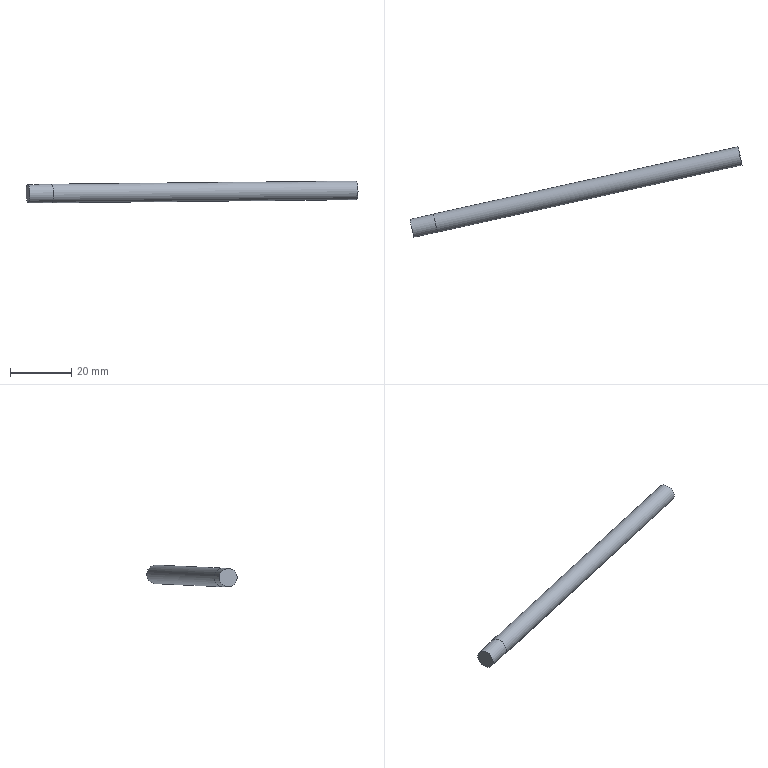Part | NX | features 9416K301(shaft) 2 | 1 solid | 5 faces | box 108.548 x 29.547 x 7.145 mm | volume 3198 mm3 | plane 3 | cylinder 2 | commonest cylinder face diameters 6 x1 6.096 x1
STEP:
#1=CARTESIAN_POINT('',(274.132,-69.062,-85.091));
#2=VERTEX_POINT('',#1);
#3=CARTESIAN_POINT('',(274.161,-69.055,-88.09));
#4=DIRECTION('',(-0.9765,-0.2153,-0.009994));
#5=DIRECTION('',(-0.009759,-0.002151,1.));
#6=AXIS2_PLACEMENT_3D('',#3,#4,#5);
#7=CIRCLE('',#6,3.);
#8=EDGE_CURVE('',#2,#2,#7,.T.);
#9=ORIENTED_EDGE('',*,*,#8,.F.);
#10=EDGE_LOOP('',(#9));
#11=FACE_BOUND('',#10,.T.);
#12=CARTESIAN_POINT('',(281.821,-67.367,-85.012));
#13=VERTEX_POINT('',#12);
#14=CARTESIAN_POINT('',(281.85,-67.36,-88.012));
#15=DIRECTION('',(-0.9765,-0.2153,-0.009994));
#16=DIRECTION('',(-0.009759,-0.002151,1.));
#17=AXIS2_PLACEMENT_3D('',#14,#15,#16);
#18=CIRCLE('',#17,3.);
#19=EDGE_CURVE('',#13,#13,#18,.T.);
#20=ORIENTED_EDGE('',*,*,#19,.T.);
#21=EDGE_LOOP('',(#20));
#22=FACE_BOUND('',#21,.T.);
#23=CARTESIAN_POINT('',(281.85,-67.36,-88.012));
#24=DIRECTION('',(-0.9765,-0.2153,-0.009994));
#25=DIRECTION('',(-0.009759,-0.002151,1.));
#26=AXIS2_PLACEMENT_3D('',#23,#24,#25);
#27=CYLINDRICAL_SURFACE('',#26,3.);
#28=ADVANCED_FACE('',(#11,#22),#27,.T.);
#29=ORIENTED_EDGE('',*,*,#8,.T.);
#30=EDGE_LOOP('',(#29));
#31=FACE_BOUND('',#30,.T.);
#32=CARTESIAN_POINT('',(274.161,-69.055,-88.09));
#33=DIRECTION('',(0.9765,0.2153,0.009994));
#34=DIRECTION('',(0.009759,0.002151,-1.));
#35=AXIS2_PLACEMENT_3D('',#32,#33,#34);
#36=PLANE('',#35);
#37=ADVANCED_FACE('',(#31),#36,.F.);
#38=ORIENTED_EDGE('',*,*,#19,.F.);
#39=EDGE_LOOP('',(#38));
#40=FACE_BOUND('',#39,.T.);
#41=CARTESIAN_POINT('',(281.88,-67.354,-91.06));
#42=VERTEX_POINT('',#41);
#43=CARTESIAN_POINT('',(281.85,-67.36,-88.012));
#44=DIRECTION('',(0.9765,0.2153,0.009994));
#45=DIRECTION('',(0.009759,0.002151,-1.));
#46=AXIS2_PLACEMENT_3D('',#43,#44,#45);
#47=CIRCLE('',#46,3.048);
#48=EDGE_CURVE('',#42,#42,#47,.T.);
#49=ORIENTED_EDGE('',*,*,#48,.F.);
#50=EDGE_LOOP('',(#49));
#51=FACE_BOUND('',#50,.T.);
#52=CARTESIAN_POINT('',(281.85,-67.36,-88.012));
#53=DIRECTION('',(-0.9765,-0.2153,-0.009994));
#54=DIRECTION('',(-0.009759,-0.002151,1.));
#55=AXIS2_PLACEMENT_3D('',#52,#53,#54);
#56=PLANE('',#55);
#57=ADVANCED_FACE('',(#40,#51),#56,.T.);
#58=ORIENTED_EDGE('',*,*,#48,.T.);
#59=EDGE_LOOP('',(#58));
#60=FACE_BOUND('',#59,.T.);
#61=CARTESIAN_POINT('',(380.75,-42.438,-86.993));
#62=VERTEX_POINT('',#61);
#63=CARTESIAN_POINT('',(381.406,-45.415,-86.993));
#64=DIRECTION('',(0.9765,0.2153,0.009994));
#65=DIRECTION('',(-0.2153,0.9766,0.));
#66=AXIS2_PLACEMENT_3D('',#63,#64,#65);
#67=CIRCLE('',#66,3.048);
#68=EDGE_CURVE('',#62,#62,#67,.T.);
#69=ORIENTED_EDGE('',*,*,#68,.F.);
#70=EDGE_LOOP('',(#69));
#71=FACE_BOUND('',#70,.T.);
#72=CARTESIAN_POINT('',(281.85,-67.36,-88.012));
#73=DIRECTION('',(0.9765,0.2153,0.009994));
#74=DIRECTION('',(0.009759,0.002151,-1.));
#75=AXIS2_PLACEMENT_3D('',#72,#73,#74);
#76=CYLINDRICAL_SURFACE('',#75,3.048);
#77=ADVANCED_FACE('',(#60,#71),#76,.T.);
#78=ORIENTED_EDGE('',*,*,#68,.T.);
#79=EDGE_LOOP('',(#78));
#80=FACE_BOUND('',#79,.T.);
#81=CARTESIAN_POINT('',(381.436,-45.408,-90.041));
#82=DIRECTION('',(0.9765,0.2153,0.009994));
#83=DIRECTION('',(0.009759,0.002151,-1.));
#84=AXIS2_PLACEMENT_3D('',#81,#82,#83);
#85=PLANE('',#84);
#86=ADVANCED_FACE('',(#80),#85,.T.);
#87=CLOSED_SHELL('',(#28,#37,#57,#77,#86));
#88=MANIFOLD_SOLID_BREP('',#87);
#89=(LENGTH_UNIT()NAMED_UNIT(*)SI_UNIT(.MILLI.,.METRE.));
#90=UNCERTAINTY_MEASURE_WITH_UNIT(LENGTH_MEASURE(0.00001),#89,'','');
#91=(NAMED_UNIT(*)PLANE_ANGLE_UNIT()SI_UNIT($,.RADIAN.));
#92=(NAMED_UNIT(*)SI_UNIT($,.STERADIAN.)SOLID_ANGLE_UNIT());
#93=(GEOMETRIC_REPRESENTATION_CONTEXT(3)GLOBAL_UNCERTAINTY_ASSIGNED_CONTEXT((#90))GLOBAL_UNIT_ASSIGNED_CONTEXT((#89,#91,#92))REPRESENTATION_CONTEXT('',''));
#94=ADVANCED_BREP_SHAPE_REPRESENTATION('',(#88),#93);